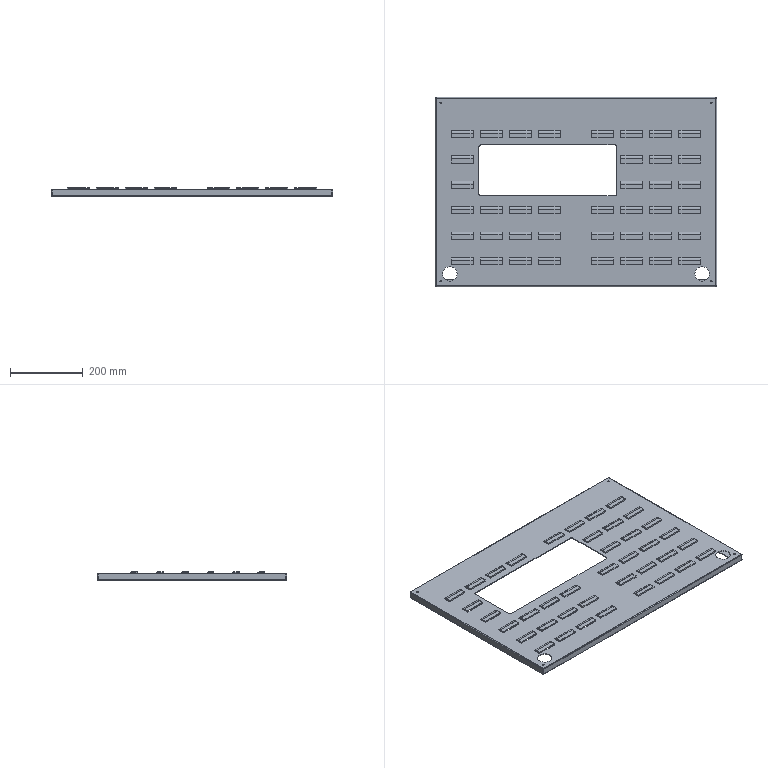Part | STEP file | 11-FG-JX01611 | 1 solid | 464 faces | box 775 x 521 x 24.03 mm | volume 906085 mm3 | plane 340 | cylinder 116 | sphere 8 | commonest cylinder face diameters 12.441 x40 16.441 x40 4.5 x16 4 x12 10 x4 40 x4